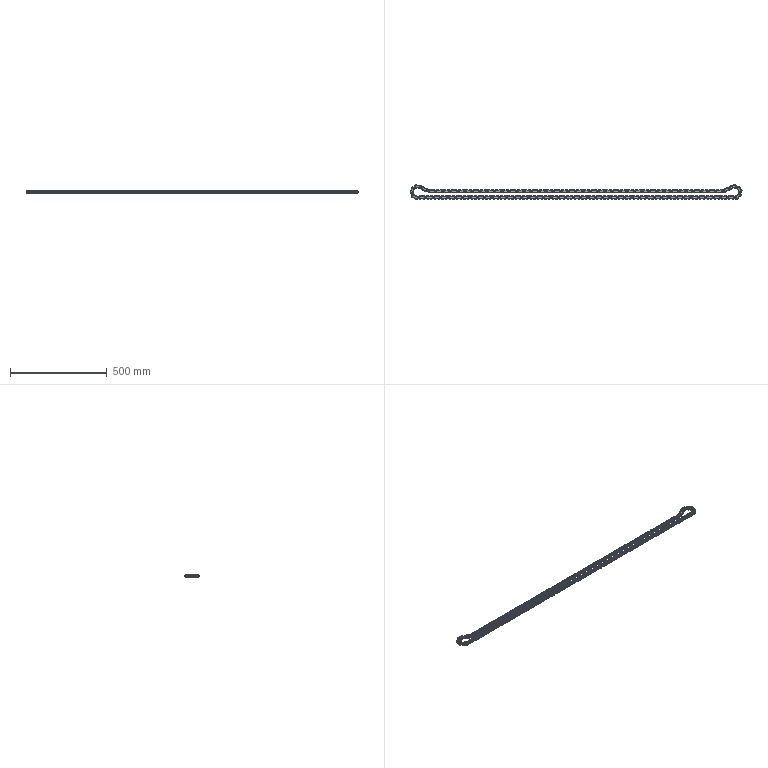Part | STEP file | MYT-A01-P03 | 91 solids | 5824 faces | volume 527480 mm3 | torus 2184 | plane 1820 | cylinder 1820 | commonest cylinder face diameters 11.91 x728 3.28 x364 8.8 x364 18.3 x364